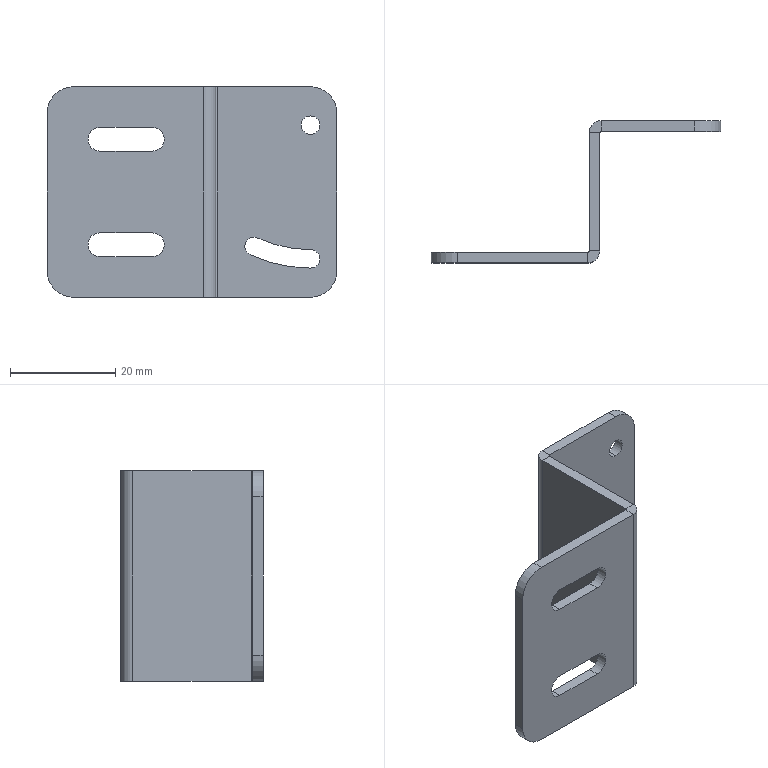Part | SolidWorks | features ICE 2, Fillet 1, FlatPattern 1, SMBaseFlange 1, SheetMetal 1 | 1 solid | 41 faces | box 55 x 27 x 40 mm | volume 5908 mm3 | plane 22 | cylinder 19 | commonest cylinder face diameters 3.5 x5 4.5 x4 10 x4 0.6 x2 4.6 x2 47.3 x1
STEP:
#1=CARTESIAN_POINT('',(20.,23.,30.95));
#2=VERTEX_POINT('',#1);
#3=CARTESIAN_POINT('',(20.,23.,34.45));
#4=VERTEX_POINT('',#3);
#5=CARTESIAN_POINT('',(20.,23.,32.7));
#6=DIRECTION('',(0.,1.,0.));
#7=DIRECTION('',(0.,0.,1.));
#8=AXIS2_PLACEMENT_3D('',#5,#6,#7);
#9=CIRCLE('',#8,1.75);
#10=EDGE_CURVE('',#2,#4,#9,.T.);
#11=ORIENTED_EDGE('',*,*,#10,.F.);
#12=CARTESIAN_POINT('',(20.,25.,30.95));
#13=VERTEX_POINT('',#12);
#14=CARTESIAN_POINT('',(20.,15.,30.95));
#15=DIRECTION('',(0.,1.,0.));
#16=VECTOR('',#15,1000.);
#17=LINE('',#14,#16);
#18=EDGE_CURVE('',#2,#13,#17,.T.);
#19=ORIENTED_EDGE('',*,*,#18,.T.);
#20=CARTESIAN_POINT('',(20.,25.,34.45));
#21=VERTEX_POINT('',#20);
#22=CARTESIAN_POINT('',(20.,25.,32.7));
#23=DIRECTION('',(0.,1.,0.));
#24=DIRECTION('',(0.,0.,1.));
#25=AXIS2_PLACEMENT_3D('',#22,#23,#24);
#26=CIRCLE('',#25,1.75);
#27=EDGE_CURVE('',#13,#21,#26,.T.);
#28=ORIENTED_EDGE('',*,*,#27,.T.);
#29=CARTESIAN_POINT('',(20.,15.,34.45));
#30=DIRECTION('',(0.,1.,0.));
#31=VECTOR('',#30,1000.);
#32=LINE('',#29,#31);
#33=EDGE_CURVE('',#4,#21,#32,.T.);
#34=ORIENTED_EDGE('',*,*,#33,.F.);
#35=EDGE_LOOP('',(#11,#19,#28,#34));
#36=FACE_OUTER_BOUND('',#35,.T.);
#37=CARTESIAN_POINT('',(20.,15.,32.7));
#38=DIRECTION('',(0.,1.,0.));
#39=DIRECTION('',(0.,0.,1.));
#40=AXIS2_PLACEMENT_3D('',#37,#38,#39);
#41=CYLINDRICAL_SURFACE('',#40,1.75);
#42=ADVANCED_FACE('',(#36),#41,.F.);
#43=CARTESIAN_POINT('',(9.265,23.,11.43));
#44=VERTEX_POINT('',#43);
#45=CARTESIAN_POINT('',(10.005,23.,11.266));
#46=VERTEX_POINT('',#45);
#47=CARTESIAN_POINT('',(9.265,23.,9.68));
#48=DIRECTION('',(0.,1.,0.));
#49=DIRECTION('',(0.,0.,1.));
#50=AXIS2_PLACEMENT_3D('',#47,#48,#49);
#51=CIRCLE('',#50,1.75);
#52=EDGE_CURVE('',#44,#46,#51,.T.);
#53=ORIENTED_EDGE('',*,*,#52,.F.);
#54=CARTESIAN_POINT('',(9.265,25.,11.43));
#55=VERTEX_POINT('',#54);
#56=CARTESIAN_POINT('',(9.265,15.,11.43));
#57=DIRECTION('',(0.,1.,0.));
#58=VECTOR('',#57,1000.);
#59=LINE('',#56,#58);
#60=EDGE_CURVE('',#44,#55,#59,.T.);
#61=ORIENTED_EDGE('',*,*,#60,.T.);
#62=CARTESIAN_POINT('',(10.005,25.,11.266));
#63=VERTEX_POINT('',#62);
#64=CARTESIAN_POINT('',(9.265,25.,9.68));
#65=DIRECTION('',(0.,1.,0.));
#66=DIRECTION('',(0.,0.,1.));
#67=AXIS2_PLACEMENT_3D('',#64,#65,#66);
#68=CIRCLE('',#67,1.75);
#69=EDGE_CURVE('',#55,#63,#68,.T.);
#70=ORIENTED_EDGE('',*,*,#69,.T.);
#71=CARTESIAN_POINT('',(10.005,15.,11.266));
#72=DIRECTION('',(0.,1.,0.));
#73=VECTOR('',#72,1000.);
#74=LINE('',#71,#73);
#75=EDGE_CURVE('',#46,#63,#74,.T.);
#76=ORIENTED_EDGE('',*,*,#75,.F.);
#77=EDGE_LOOP('',(#53,#61,#70,#76));
#78=FACE_OUTER_BOUND('',#77,.T.);
#79=CARTESIAN_POINT('',(9.265,15.,9.68));
#80=DIRECTION('',(0.,1.,0.));
#81=DIRECTION('',(0.,0.,1.));
#82=AXIS2_PLACEMENT_3D('',#79,#80,#81);
#83=CYLINDRICAL_SURFACE('',#82,1.75);
#84=ADVANCED_FACE('',(#78),#83,.F.);
#85=CARTESIAN_POINT('',(0.,0.3,40.));
#86=VERTEX_POINT('',#85);
#87=CARTESIAN_POINT('',(2.,0.3,40.));
#88=VERTEX_POINT('',#87);
#89=CARTESIAN_POINT('',(0.,0.3,40.));
#90=DIRECTION('',(1.,0.,0.));
#91=VECTOR('',#90,1000.);
#92=LINE('',#89,#91);
#93=EDGE_CURVE('',#86,#88,#92,.T.);
#94=ORIENTED_EDGE('',*,*,#93,.F.);
#95=CARTESIAN_POINT('',(-0.3,0.,40.));
#96=VERTEX_POINT('',#95);
#97=CARTESIAN_POINT('',(-0.3,0.3,40.));
#98=DIRECTION('',(0.,0.,1.));
#99=DIRECTION('',(-1.,0.,0.));
#100=AXIS2_PLACEMENT_3D('',#97,#98,#99);
#101=CIRCLE('',#100,0.3);
#102=EDGE_CURVE('',#96,#86,#101,.T.);
#103=ORIENTED_EDGE('',*,*,#102,.F.);
#104=CARTESIAN_POINT('',(-0.3,-2.,40.));
#105=VERTEX_POINT('',#104);
#106=CARTESIAN_POINT('',(-0.3,-2.,40.));
#107=DIRECTION('',(0.,1.,0.));
#108=VECTOR('',#107,1000.);
#109=LINE('',#106,#108);
#110=EDGE_CURVE('',#105,#96,#109,.T.);
#111=ORIENTED_EDGE('',*,*,#110,.F.);
#112=CARTESIAN_POINT('',(-0.3,0.3,40.));
#113=DIRECTION('',(0.,0.,1.));
#114=DIRECTION('',(1.,0.,0.));
#115=AXIS2_PLACEMENT_3D('',#112,#113,#114);
#116=CIRCLE('',#115,2.3);
#117=EDGE_CURVE('',#105,#88,#116,.T.);
#118=ORIENTED_EDGE('',*,*,#117,.T.);
#119=EDGE_LOOP('',(#94,#103,#111,#118));
#120=FACE_OUTER_BOUND('',#119,.T.);
#121=CARTESIAN_POINT('',(0.,0.3,40.));
#122=DIRECTION('',(0.,0.,1.));
#123=DIRECTION('',(1.,0.,0.));
#124=AXIS2_PLACEMENT_3D('',#121,#122,#123);
#125=PLANE('',#124);
#126=ADVANCED_FACE('',(#120),#125,.T.);
#127=CARTESIAN_POINT('',(0.,22.7,40.));
#128=VERTEX_POINT('',#127);
#129=CARTESIAN_POINT('',(0.,0.,40.));
#130=DIRECTION('',(0.,1.,0.));
#131=VECTOR('',#130,1000.);
#132=LINE('',#129,#131);
#133=EDGE_CURVE('',#86,#128,#132,.T.);
#134=ORIENTED_EDGE('',*,*,#133,.F.);
#135=ORIENTED_EDGE('',*,*,#93,.T.);
#136=CARTESIAN_POINT('',(2.,22.7,40.));
#137=VERTEX_POINT('',#136);
#138=CARTESIAN_POINT('',(2.,0.,40.));
#139=DIRECTION('',(0.,1.,0.));
#140=VECTOR('',#139,1000.);
#141=LINE('',#138,#140);
#142=EDGE_CURVE('',#88,#137,#141,.T.);
#143=ORIENTED_EDGE('',*,*,#142,.T.);
#144=CARTESIAN_POINT('',(2.,22.7,40.));
#145=DIRECTION('',(-1.,0.,0.));
#146=VECTOR('',#145,1000.);
#147=LINE('',#144,#146);
#148=EDGE_CURVE('',#137,#128,#147,.T.);
#149=ORIENTED_EDGE('',*,*,#148,.T.);
#150=EDGE_LOOP('',(#134,#135,#143,#149));
#151=FACE_OUTER_BOUND('',#150,.T.);
#152=CARTESIAN_POINT('',(-0.3,-2.,40.));
#153=DIRECTION('',(0.,0.,1.));
#154=DIRECTION('',(1.,0.,0.));
#155=AXIS2_PLACEMENT_3D('',#152,#153,#154);
#156=PLANE('',#155);
#157=ADVANCED_FACE('',(#151),#156,.T.);
#158=CARTESIAN_POINT('',(-0.3,0.,0.));
#159=VERTEX_POINT('',#158);
#160=CARTESIAN_POINT('',(-0.3,-2.,0.));
#161=VERTEX_POINT('',#160);
#162=CARTESIAN_POINT('',(-0.3,0.,0.));
#163=DIRECTION('',(0.,-1.,0.));
#164=VECTOR('',#163,1000.);
#165=LINE('',#162,#164);
#166=EDGE_CURVE('',#159,#161,#165,.T.);
#167=ORIENTED_EDGE('',*,*,#166,.F.);
#168=CARTESIAN_POINT('',(0.,0.3,0.));
#169=VERTEX_POINT('',#168);
#170=CARTESIAN_POINT('',(-0.3,0.3,0.));
#171=DIRECTION('',(0.,0.,1.));
#172=DIRECTION('',(-1.,0.,0.));
#173=AXIS2_PLACEMENT_3D('',#170,#171,#172);
#174=CIRCLE('',#173,0.3);
#175=EDGE_CURVE('',#159,#169,#174,.T.);
#176=ORIENTED_EDGE('',*,*,#175,.T.);
#177=CARTESIAN_POINT('',(2.,0.3,0.));
#178=VERTEX_POINT('',#177);
#179=CARTESIAN_POINT('',(2.,0.3,0.));
#180=DIRECTION('',(-1.,0.,0.));
#181=VECTOR('',#180,1000.);
#182=LINE('',#179,#181);
#183=EDGE_CURVE('',#178,#169,#182,.T.);
#184=ORIENTED_EDGE('',*,*,#183,.F.);
#185=CARTESIAN_POINT('',(-0.3,0.3,0.));
#186=DIRECTION('',(0.,0.,1.));
#187=DIRECTION('',(1.,0.,0.));
#188=AXIS2_PLACEMENT_3D('',#185,#186,#187);
#189=CIRCLE('',#188,2.3);
#190=EDGE_CURVE('',#161,#178,#189,.T.);
#191=ORIENTED_EDGE('',*,*,#190,.F.);
#192=EDGE_LOOP('',(#167,#176,#184,#191));
#193=FACE_OUTER_BOUND('',#192,.T.);
#194=CARTESIAN_POINT('',(-0.3,0.,0.));
#195=DIRECTION('',(0.,0.,-1.));
#196=DIRECTION('',(-1.,0.,0.));
#197=AXIS2_PLACEMENT_3D('',#194,#195,#196);
#198=PLANE('',#197);
#199=ADVANCED_FACE('',(#193),#198,.T.);
#200=CARTESIAN_POINT('',(-25.,-2.,0.));
#201=VERTEX_POINT('',#200);
#202=CARTESIAN_POINT('',(-30.,-2.,0.));
#203=DIRECTION('',(1.,0.,0.));
#204=VECTOR('',#203,1000.);
#205=LINE('',#202,#204);
#206=EDGE_CURVE('',#201,#161,#205,.T.);
#207=ORIENTED_EDGE('',*,*,#206,.F.);
#208=CARTESIAN_POINT('',(-25.,0.,0.));
#209=VERTEX_POINT('',#208);
#210=CARTESIAN_POINT('',(-25.,0.3,0.));
#211=DIRECTION('',(0.,1.,0.));
#212=VECTOR('',#211,1000.);
#213=LINE('',#210,#212);
#214=EDGE_CURVE('',#201,#209,#213,.T.);
#215=ORIENTED_EDGE('',*,*,#214,.T.);
#216=CARTESIAN_POINT('',(-30.,0.,0.));
#217=DIRECTION('',(1.,0.,0.));
#218=VECTOR('',#217,1000.);
#219=LINE('',#216,#218);
#220=EDGE_CURVE('',#209,#159,#219,.T.);
#221=ORIENTED_EDGE('',*,*,#220,.T.);
#222=ORIENTED_EDGE('',*,*,#166,.T.);
#223=EDGE_LOOP('',(#207,#215,#221,#222));
#224=FACE_OUTER_BOUND('',#223,.T.);
#225=CARTESIAN_POINT('',(2.,0.3,0.));
#226=DIRECTION('',(0.,0.,-1.));
#227=DIRECTION('',(-1.,0.,0.));
#228=AXIS2_PLACEMENT_3D('',#225,#226,#227);
#229=PLANE('',#228);
#230=ADVANCED_FACE('',(#224),#229,.T.);
#231=CARTESIAN_POINT('',(2.3,25.,40.));
#232=VERTEX_POINT('',#231);
#233=CARTESIAN_POINT('',(2.3,23.,40.));
#234=VERTEX_POINT('',#233);
#235=CARTESIAN_POINT('',(2.3,25.,40.));
#236=DIRECTION('',(0.,-1.,0.));
#237=VECTOR('',#236,1000.);
#238=LINE('',#235,#237);
#239=EDGE_CURVE('',#232,#234,#238,.T.);
#240=ORIENTED_EDGE('',*,*,#239,.F.);
#241=CARTESIAN_POINT('',(2.3,22.7,40.));
#242=DIRECTION('',(0.,0.,-1.));
#243=DIRECTION('',(1.,0.,0.));
#244=AXIS2_PLACEMENT_3D('',#241,#242,#243);
#245=CIRCLE('',#244,2.3);
#246=EDGE_CURVE('',#128,#232,#245,.T.);
#247=ORIENTED_EDGE('',*,*,#246,.F.);
#248=ORIENTED_EDGE('',*,*,#148,.F.);
#249=CARTESIAN_POINT('',(2.3,22.7,40.));
#250=DIRECTION('',(0.,0.,-1.));
#251=DIRECTION('',(1.,0.,0.));
#252=AXIS2_PLACEMENT_3D('',#249,#250,#251);
#253=CIRCLE('',#252,0.3);
#254=EDGE_CURVE('',#137,#234,#253,.T.);
#255=ORIENTED_EDGE('',*,*,#254,.T.);
#256=EDGE_LOOP('',(#240,#247,#248,#255));
#257=FACE_OUTER_BOUND('',#256,.T.);
#258=CARTESIAN_POINT('',(2.3,25.,40.));
#259=DIRECTION('',(0.,0.,1.));
#260=DIRECTION('',(1.,0.,0.));
#261=AXIS2_PLACEMENT_3D('',#258,#259,#260);
#262=PLANE('',#261);
#263=ADVANCED_FACE('',(#257),#262,.T.);
#264=CARTESIAN_POINT('',(20.,23.,40.));
#265=VERTEX_POINT('',#264);
#266=CARTESIAN_POINT('',(0.,23.,40.));
#267=DIRECTION('',(1.,0.,0.));
#268=VECTOR('',#267,1000.);
#269=LINE('',#266,#268);
#270=EDGE_CURVE('',#234,#265,#269,.T.);
#271=ORIENTED_EDGE('',*,*,#270,.T.);
#272=CARTESIAN_POINT('',(20.,25.,40.));
#273=VERTEX_POINT('',#272);
#274=CARTESIAN_POINT('',(20.,22.7,40.));
#275=DIRECTION('',(0.,1.,0.));
#276=VECTOR('',#275,1000.);
#277=LINE('',#274,#276);
#278=EDGE_CURVE('',#265,#273,#277,.T.);
#279=ORIENTED_EDGE('',*,*,#278,.T.);
#280=CARTESIAN_POINT('',(0.,25.,40.));
#281=DIRECTION('',(1.,0.,0.));
#282=VECTOR('',#281,1000.);
#283=LINE('',#280,#282);
#284=EDGE_CURVE('',#232,#273,#283,.T.);
#285=ORIENTED_EDGE('',*,*,#284,.F.);
#286=ORIENTED_EDGE('',*,*,#239,.T.);
#287=EDGE_LOOP('',(#271,#279,#285,#286));
#288=FACE_OUTER_BOUND('',#287,.T.);
#289=CARTESIAN_POINT('',(2.,22.7,40.));
#290=DIRECTION('',(0.,0.,1.));
#291=DIRECTION('',(1.,0.,0.));
#292=AXIS2_PLACEMENT_3D('',#289,#290,#291);
#293=PLANE('',#292);
#294=ADVANCED_FACE('',(#288),#293,.T.);
#295=CARTESIAN_POINT('',(0.,22.7,0.));
#296=VERTEX_POINT('',#295);
#297=CARTESIAN_POINT('',(2.,22.7,0.));
#298=VERTEX_POINT('',#297);
#299=CARTESIAN_POINT('',(0.,22.7,0.));
#300=DIRECTION('',(1.,0.,0.));
#301=VECTOR('',#300,1000.);
#302=LINE('',#299,#301);
#303=EDGE_CURVE('',#296,#298,#302,.T.);
#304=ORIENTED_EDGE('',*,*,#303,.F.);
#305=CARTESIAN_POINT('',(2.3,25.,0.));
#306=VERTEX_POINT('',#305);
#307=CARTESIAN_POINT('',(2.3,22.7,0.));
#308=DIRECTION('',(0.,0.,-1.));
#309=DIRECTION('',(1.,0.,0.));
#310=AXIS2_PLACEMENT_3D('',#307,#308,#309);
#311=CIRCLE('',#310,2.3);
#312=EDGE_CURVE('',#296,#306,#311,.T.);
#313=ORIENTED_EDGE('',*,*,#312,.T.);
#314=CARTESIAN_POINT('',(2.3,23.,0.));
#315=VERTEX_POINT('',#314);
#316=CARTESIAN_POINT('',(2.3,23.,0.));
#317=DIRECTION('',(0.,1.,0.));
#318=VECTOR('',#317,1000.);
#319=LINE('',#316,#318);
#320=EDGE_CURVE('',#315,#306,#319,.T.);
#321=ORIENTED_EDGE('',*,*,#320,.F.);
#322=CARTESIAN_POINT('',(2.3,22.7,0.));
#323=DIRECTION('',(0.,0.,-1.));
#324=DIRECTION('',(1.,0.,0.));
#325=AXIS2_PLACEMENT_3D('',#322,#323,#324);
#326=CIRCLE('',#325,0.3);
#327=EDGE_CURVE('',#298,#315,#326,.T.);
#328=ORIENTED_EDGE('',*,*,#327,.F.);
#329=EDGE_LOOP('',(#304,#313,#321,#328));
#330=FACE_OUTER_BOUND('',#329,.T.);
#331=CARTESIAN_POINT('',(0.,22.7,0.));
#332=DIRECTION('',(0.,0.,-1.));
#333=DIRECTION('',(-1.,0.,0.));
#334=AXIS2_PLACEMENT_3D('',#331,#332,#333);
#335=PLANE('',#334);
#336=ADVANCED_FACE('',(#330),#335,.T.);
#337=CARTESIAN_POINT('',(0.,0.,0.));
#338=DIRECTION('',(0.,1.,0.));
#339=VECTOR('',#338,1000.);
#340=LINE('',#337,#339);
#341=EDGE_CURVE('',#169,#296,#340,.T.);
#342=ORIENTED_EDGE('',*,*,#341,.T.);
#343=ORIENTED_EDGE('',*,*,#303,.T.);
#344=CARTESIAN_POINT('',(2.,0.,0.));
#345=DIRECTION('',(0.,1.,0.));
#346=VECTOR('',#345,1000.);
#347=LINE('',#344,#346);
#348=EDGE_CURVE('',#178,#298,#347,.T.);
#349=ORIENTED_EDGE('',*,*,#348,.F.);
#350=ORIENTED_EDGE('',*,*,#183,.T.);
#351=EDGE_LOOP('',(#342,#343,#349,#350));
#352=FACE_OUTER_BOUND('',#351,.T.);
#353=CARTESIAN_POINT('',(2.3,23.,0.));
#354=DIRECTION('',(0.,0.,-1.));
#355=DIRECTION('',(-1.,0.,0.));
#356=AXIS2_PLACEMENT_3D('',#353,#354,#355);
#357=PLANE('',#356);
#358=ADVANCED_FACE('',(#352),#357,.T.);
#359=CARTESIAN_POINT('',(20.,23.,32.7));
#360=DIRECTION('',(0.,1.,0.));
#361=DIRECTION('',(0.,0.,1.));
#362=AXIS2_PLACEMENT_3D('',#359,#360,#361);
#363=CIRCLE('',#362,1.75);
#364=EDGE_CURVE('',#4,#2,#363,.T.);
#365=ORIENTED_EDGE('',*,*,#364,.T.);
#366=ORIENTED_EDGE('',*,*,#10,.T.);
#367=EDGE_LOOP('',(#365,#366));
#368=FACE_BOUND('',#367,.T.);
#369=CARTESIAN_POINT('',(20.,23.,9.05));
#370=VERTEX_POINT('',#369);
#371=CARTESIAN_POINT('',(20.,23.,32.7));
#372=DIRECTION('',(0.,-1.,0.));
#373=DIRECTION('',(0.,0.,1.));
#374=AXIS2_PLACEMENT_3D('',#371,#372,#373);
#375=CIRCLE('',#374,23.65);
#376=EDGE_CURVE('',#46,#370,#375,.T.);
#377=ORIENTED_EDGE('',*,*,#376,.T.);
#378=CARTESIAN_POINT('',(20.,23.,5.55));
#379=VERTEX_POINT('',#378);
#380=CARTESIAN_POINT('',(20.,23.,7.3));
#381=DIRECTION('',(0.,1.,0.));
#382=DIRECTION('',(0.,0.,1.));
#383=AXIS2_PLACEMENT_3D('',#380,#381,#382);
#384=CIRCLE('',#383,1.75);
#385=EDGE_CURVE('',#370,#379,#384,.T.);
#386=ORIENTED_EDGE('',*,*,#385,.T.);
#387=CARTESIAN_POINT('',(8.526,23.,8.094));
#388=VERTEX_POINT('',#387);
#389=CARTESIAN_POINT('',(20.,23.,32.7));
#390=DIRECTION('',(0.,1.,0.));
#391=DIRECTION('',(0.,0.,1.));
#392=AXIS2_PLACEMENT_3D('',#389,#390,#391);
#393=CIRCLE('',#392,27.15);
#394=EDGE_CURVE('',#379,#388,#393,.T.);
#395=ORIENTED_EDGE('',*,*,#394,.T.);
#396=CARTESIAN_POINT('',(9.265,23.,9.68));
#397=DIRECTION('',(0.,1.,0.));
#398=DIRECTION('',(0.,0.,1.));
#399=AXIS2_PLACEMENT_3D('',#396,#397,#398);
#400=CIRCLE('',#399,1.75);
#401=EDGE_CURVE('',#388,#44,#400,.T.);
#402=ORIENTED_EDGE('',*,*,#401,.T.);
#403=ORIENTED_EDGE('',*,*,#52,.T.);
#404=EDGE_LOOP('',(#377,#386,#395,#402,#403));
#405=FACE_BOUND('',#404,.T.);
#406=CARTESIAN_POINT('',(25.,23.,35.));
#407=VERTEX_POINT('',#406);
#408=CARTESIAN_POINT('',(25.,23.,5.));
#409=VERTEX_POINT('',#408);
#410=CARTESIAN_POINT('',(25.,23.,40.));
#411=DIRECTION('',(0.,0.,-1.));
#412=VECTOR('',#411,1000.);
#413=LINE('',#410,#412);
#414=EDGE_CURVE('',#407,#409,#413,.T.);
#415=ORIENTED_EDGE('',*,*,#414,.F.);
#416=CARTESIAN_POINT('',(20.,23.,35.));
#417=DIRECTION('',(0.,-1.,0.));
#418=DIRECTION('',(0.,0.,1.));
#419=AXIS2_PLACEMENT_3D('',#416,#417,#418);
#420=CIRCLE('',#419,5.);
#421=EDGE_CURVE('',#407,#265,#420,.T.);
#422=ORIENTED_EDGE('',*,*,#421,.T.);
#423=ORIENTED_EDGE('',*,*,#270,.F.);
#424=CARTESIAN_POINT('',(2.3,23.,40.));
#425=DIRECTION('',(0.,0.,-1.));
#426=VECTOR('',#425,1000.);
#427=LINE('',#424,#426);
#428=EDGE_CURVE('',#234,#315,#427,.T.);
#429=ORIENTED_EDGE('',*,*,#428,.T.);
#430=CARTESIAN_POINT('',(20.,23.,0.));
#431=VERTEX_POINT('',#430);
#432=CARTESIAN_POINT('',(0.,23.,0.));
#433=DIRECTION('',(1.,0.,0.));
#434=VECTOR('',#433,1000.);
#435=LINE('',#432,#434);
#436=EDGE_CURVE('',#315,#431,#435,.T.);
#437=ORIENTED_EDGE('',*,*,#436,.T.);
#438=CARTESIAN_POINT('',(20.,23.,5.));
#439=DIRECTION('',(0.,-1.,0.));
#440=DIRECTION('',(0.,0.,1.));
#441=AXIS2_PLACEMENT_3D('',#438,#439,#440);
#442=CIRCLE('',#441,5.);
#443=EDGE_CURVE('',#431,#409,#442,.T.);
#444=ORIENTED_EDGE('',*,*,#443,.T.);
#445=EDGE_LOOP('',(#415,#422,#423,#429,#437,#444));
#446=FACE_OUTER_BOUND('',#445,.T.);
#447=CARTESIAN_POINT('',(0.,23.,40.));
#448=DIRECTION('',(0.,1.,0.));
#449=DIRECTION('',(0.,0.,1.));
#450=AXIS2_PLACEMENT_3D('',#447,#448,#449);
#451=PLANE('',#450);
#452=ADVANCED_FACE('',(#368,#405,#446),#451,.F.);
#453=CARTESIAN_POINT('',(25.,25.,35.));
#454=VERTEX_POINT('',#453);
#455=CARTESIAN_POINT('',(25.,25.,5.));
#456=VERTEX_POINT('',#455);
#457=CARTESIAN_POINT('',(25.,25.,40.));
#458=DIRECTION('',(0.,0.,-1.));
#459=VECTOR('',#458,1000.);
#460=LINE('',#457,#459);
#461=EDGE_CURVE('',#454,#456,#460,.T.);
#462=ORIENTED_EDGE('',*,*,#461,.F.);
#463=CARTESIAN_POINT('',(25.,25.,35.));
#464=DIRECTION('',(0.,-1.,0.));
#465=VECTOR('',#464,1000.);
#466=LINE('',#463,#465);
#467=EDGE_CURVE('',#454,#407,#466,.T.);
#468=ORIENTED_EDGE('',*,*,#467,.T.);
#469=ORIENTED_EDGE('',*,*,#414,.T.);
#470=CARTESIAN_POINT('',(25.,25.,5.));
#471=DIRECTION('',(0.,1.,0.));
#472=VECTOR('',#471,1000.);
#473=LINE('',#470,#472);
#474=EDGE_CURVE('',#409,#456,#473,.T.);
#475=ORIENTED_EDGE('',*,*,#474,.T.);
#476=EDGE_LOOP('',(#462,#468,#469,#475));
#477=FACE_OUTER_BOUND('',#476,.T.);
#478=CARTESIAN_POINT('',(25.,25.,40.));
#479=DIRECTION('',(1.,0.,0.));
#480=DIRECTION('',(0.,0.,-1.));
#481=AXIS2_PLACEMENT_3D('',#478,#479,#480);
#482=PLANE('',#481);
#483=ADVANCED_FACE('',(#477),#482,.T.);
#484=CARTESIAN_POINT('',(20.,25.,32.7));
#485=DIRECTION('',(0.,1.,0.));
#486=DIRECTION('',(0.,0.,1.));
#487=AXIS2_PLACEMENT_3D('',#484,#485,#486);
#488=CIRCLE('',#487,1.75);
#489=EDGE_CURVE('',#21,#13,#488,.T.);
#490=ORIENTED_EDGE('',*,*,#489,.F.);
#491=ORIENTED_EDGE('',*,*,#27,.F.);
#492=EDGE_LOOP('',(#490,#491));
#493=FACE_BOUND('',#492,.T.);
#494=CARTESIAN_POINT('',(20.,25.,9.05));
#495=VERTEX_POINT('',#494);
#496=CARTESIAN_POINT('',(20.,25.,5.55));
#497=VERTEX_POINT('',#496);
#498=CARTESIAN_POINT('',(20.,25.,7.3));
#499=DIRECTION('',(0.,1.,0.));
#500=DIRECTION('',(0.,0.,1.));
#501=AXIS2_PLACEMENT_3D('',#498,#499,#500);
#502=CIRCLE('',#501,1.75);
#503=EDGE_CURVE('',#495,#497,#502,.T.);
#504=ORIENTED_EDGE('',*,*,#503,.F.);
#505=CARTESIAN_POINT('',(20.,25.,32.7));
#506=DIRECTION('',(0.,-1.,0.));
#507=DIRECTION('',(0.,0.,1.));
#508=AXIS2_PLACEMENT_3D('',#505,#506,#507);
#509=CIRCLE('',#508,23.65);
#510=EDGE_CURVE('',#63,#495,#509,.T.);
#511=ORIENTED_EDGE('',*,*,#510,.F.);
#512=ORIENTED_EDGE('',*,*,#69,.F.);
#513=CARTESIAN_POINT('',(8.526,25.,8.094));
#514=VERTEX_POINT('',#513);
#515=CARTESIAN_POINT('',(9.265,25.,9.68));
#516=DIRECTION('',(0.,1.,0.));
#517=DIRECTION('',(0.,0.,1.));
#518=AXIS2_PLACEMENT_3D('',#515,#516,#517);
#519=CIRCLE('',#518,1.75);
#520=EDGE_CURVE('',#514,#55,#519,.T.);
#521=ORIENTED_EDGE('',*,*,#520,.F.);
#522=CARTESIAN_POINT('',(20.,25.,32.7));
#523=DIRECTION('',(0.,1.,0.));
#524=DIRECTION('',(0.,0.,1.));
#525=AXIS2_PLACEMENT_3D('',#522,#523,#524);
#526=CIRCLE('',#525,27.15);
#527=EDGE_CURVE('',#497,#514,#526,.T.);
#528=ORIENTED_EDGE('',*,*,#527,.F.);
#529=EDGE_LOOP('',(#504,#511,#512,#521,#528));
#530=FACE_BOUND('',#529,.T.);
#531=ORIENTED_EDGE('',*,*,#284,.T.);
#532=CARTESIAN_POINT('',(20.,25.,35.));
#533=DIRECTION('',(0.,1.,0.));
#534=DIRECTION('',(0.,0.,1.));
#535=AXIS2_PLACEMENT_3D('',#532,#533,#534);
#536=CIRCLE('',#535,5.);
#537=EDGE_CURVE('',#273,#454,#536,.T.);
#538=ORIENTED_EDGE('',*,*,#537,.T.);
#539=ORIENTED_EDGE('',*,*,#461,.T.);
#540=CARTESIAN_POINT('',(20.,25.,0.));
#541=VERTEX_POINT('',#540);
#542=CARTESIAN_POINT('',(20.,25.,5.));
#543=DIRECTION('',(0.,1.,0.));
#544=DIRECTION('',(0.,0.,1.));
#545=AXIS2_PLACEMENT_3D('',#542,#543,#544);
#546=CIRCLE('',#545,5.);
#547=EDGE_CURVE('',#456,#541,#546,.T.);
#548=ORIENTED_EDGE('',*,*,#547,.T.);
#549=CARTESIAN_POINT('',(0.,25.,0.));
#550=DIRECTION('',(1.,0.,0.));
#551=VECTOR('',#550,1000.);
#552=LINE('',#549,#551);
#553=EDGE_CURVE('',#306,#541,#552,.T.);
#554=ORIENTED_EDGE('',*,*,#553,.F.);
#555=CARTESIAN_POINT('',(2.3,25.,40.));
#556=DIRECTION('',(0.,0.,-1.));
#557=VECTOR('',#556,1000.);
#558=LINE('',#555,#557);
#559=EDGE_CURVE('',#232,#306,#558,.T.);
#560=ORIENTED_EDGE('',*,*,#559,.F.);
#561=EDGE_LOOP('',(#531,#538,#539,#548,#554,#560));
#562=FACE_OUTER_BOUND('',#561,.T.);
#563=CARTESIAN_POINT('',(0.,25.,40.));
#564=DIRECTION('',(0.,1.,0.));
#565=DIRECTION('',(0.,0.,1.));
#566=AXIS2_PLACEMENT_3D('',#563,#564,#565);
#567=PLANE('',#566);
#568=ADVANCED_FACE('',(#493,#530,#562),#567,.T.);
#569=ORIENTED_EDGE('',*,*,#312,.F.);
#570=CARTESIAN_POINT('',(0.,22.7,40.));
#571=DIRECTION('',(0.,0.,-1.));
#572=VECTOR('',#571,1000.);
#573=LINE('',#570,#572);
#574=EDGE_CURVE('',#128,#296,#573,.T.);
#575=ORIENTED_EDGE('',*,*,#574,.F.);
#576=ORIENTED_EDGE('',*,*,#246,.T.);
#577=ORIENTED_EDGE('',*,*,#559,.T.);
#578=EDGE_LOOP('',(#569,#575,#576,#577));
#579=FACE_OUTER_BOUND('',#578,.T.);
#580=CARTESIAN_POINT('',(2.3,22.7,40.));
#581=DIRECTION('',(0.,0.,-1.));
#582=DIRECTION('',(-1.,0.,0.));
#583=AXIS2_PLACEMENT_3D('',#580,#581,#582);
#584=CYLINDRICAL_SURFACE('',#583,2.3);
#585=ADVANCED_FACE('',(#579),#584,.T.);
#586=ORIENTED_EDGE('',*,*,#341,.F.);
#587=CARTESIAN_POINT('',(0.,0.3,40.));
#588=DIRECTION('',(0.,0.,-1.));
#589=VECTOR('',#588,1000.);
#590=LINE('',#587,#589);
#591=EDGE_CURVE('',#86,#169,#590,.T.);
#592=ORIENTED_EDGE('',*,*,#591,.F.);
#593=ORIENTED_EDGE('',*,*,#133,.T.);
#594=ORIENTED_EDGE('',*,*,#574,.T.);
#595=EDGE_LOOP('',(#586,#592,#593,#594));
#596=FACE_OUTER_BOUND('',#595,.T.);
#597=CARTESIAN_POINT('',(0.,0.,40.));
#598=DIRECTION('',(-1.,0.,0.));
#599=DIRECTION('',(0.,0.,1.));
#600=AXIS2_PLACEMENT_3D('',#597,#598,#599);
#601=PLANE('',#600);
#602=ADVANCED_FACE('',(#596),#601,.T.);
#603=ORIENTED_EDGE('',*,*,#175,.F.);
#604=CARTESIAN_POINT('',(-0.3,0.,40.));
#605=DIRECTION('',(0.,0.,-1.));
#606=VECTOR('',#605,1000.);
#607=LINE('',#604,#606);
#608=EDGE_CURVE('',#96,#159,#607,.T.);
#609=ORIENTED_EDGE('',*,*,#608,.F.);
#610=ORIENTED_EDGE('',*,*,#102,.T.);
#611=ORIENTED_EDGE('',*,*,#591,.T.);
#612=EDGE_LOOP('',(#603,#609,#610,#611));
#613=FACE_OUTER_BOUND('',#612,.T.);
#614=CARTESIAN_POINT('',(-0.3,0.3,40.));
#615=DIRECTION('',(0.,0.,-1.));
#616=DIRECTION('',(-1.,0.,0.));
#617=AXIS2_PLACEMENT_3D('',#614,#615,#616);
#618=CYLINDRICAL_SURFACE('',#617,0.3);
#619=ADVANCED_FACE('',(#613),#618,.F.);
#620=CARTESIAN_POINT('',(-20.,0.,7.75));
#621=VERTEX_POINT('',#620);
#622=CARTESIAN_POINT('',(-20.,0.,12.25));
#623=VERTEX_POINT('',#622);
#624=CARTESIAN_POINT('',(-20.,0.,10.));
#625=DIRECTION('',(0.,1.,0.));
#626=DIRECTION('',(0.,0.,1.));
#627=AXIS2_PLACEMENT_3D('',#624,#625,#626);
#628=CIRCLE('',#627,2.25);
#629=EDGE_CURVE('',#621,#623,#628,.T.);
#630=ORIENTED_EDGE('',*,*,#629,.F.);
#631=CARTESIAN_POINT('',(-10.,0.,7.75));
#632=VERTEX_POINT('',#631);
#633=CARTESIAN_POINT('',(-20.,0.,7.75));
#634=DIRECTION('',(-1.,0.,0.));
#635=VECTOR('',#634,1000.);
#636=LINE('',#633,#635);
#637=EDGE_CURVE('',#632,#621,#636,.T.);
#638=ORIENTED_EDGE('',*,*,#637,.F.);
#639=CARTESIAN_POINT('',(-10.,0.,12.25));
#640=VERTEX_POINT('',#639);
#641=CARTESIAN_POINT('',(-10.,0.,10.));
#642=DIRECTION('',(0.,1.,0.));
#643=DIRECTION('',(0.,0.,1.));
#644=AXIS2_PLACEMENT_3D('',#641,#642,#643);
#645=CIRCLE('',#644,2.25);
#646=EDGE_CURVE('',#640,#632,#645,.T.);
#647=ORIENTED_EDGE('',*,*,#646,.F.);
#648=CARTESIAN_POINT('',(-20.,0.,12.25));
#649=DIRECTION('',(1.,0.,0.));
#650=VECTOR('',#649,1000.);
#651=LINE('',#648,#650);
#652=EDGE_CURVE('',#623,#640,#651,.T.);
#653=ORIENTED_EDGE('',*,*,#652,.F.);
#654=EDGE_LOOP('',(#630,#638,#647,#653));
#655=FACE_BOUND('',#654,.T.);
#656=CARTESIAN_POINT('',(-20.,0.,27.75));
#657=VERTEX_POINT('',#656);
#658=CARTESIAN_POINT('',(-20.,0.,32.25));
#659=VERTEX_POINT('',#658);
#660=CARTESIAN_POINT('',(-20.,0.,30.));
#661=DIRECTION('',(0.,1.,0.));
#662=DIRECTION('',(0.,0.,1.));
#663=AXIS2_PLACEMENT_3D('',#660,#661,#662);
#664=CIRCLE('',#663,2.25);
#665=EDGE_CURVE('',#657,#659,#664,.T.);
#666=ORIENTED_EDGE('',*,*,#665,.F.);
#667=CARTESIAN_POINT('',(-10.,0.,27.75));
#668=VERTEX_POINT('',#667);
#669=CARTESIAN_POINT('',(-20.,0.,27.75));
#670=DIRECTION('',(-1.,0.,0.));
#671=VECTOR('',#670,1000.);
#672=LINE('',#669,#671);
#673=EDGE_CURVE('',#668,#657,#672,.T.);
#674=ORIENTED_EDGE('',*,*,#673,.F.);
#675=CARTESIAN_POINT('',(-10.,0.,32.25));
#676=VERTEX_POINT('',#675);
#677=CARTESIAN_POINT('',(-10.,0.,30.));
#678=DIRECTION('',(0.,1.,0.));
#679=DIRECTION('',(0.,0.,1.));
#680=AXIS2_PLACEMENT_3D('',#677,#678,#679);
#681=CIRCLE('',#680,2.25);
#682=EDGE_CURVE('',#676,#668,#681,.T.);
#683=ORIENTED_EDGE('',*,*,#682,.F.);
#684=CARTESIAN_POINT('',(-20.,0.,32.25));
#685=DIRECTION('',(1.,0.,0.));
#686=VECTOR('',#685,1000.);
#687=LINE('',#684,#686);
#688=EDGE_CURVE('',#659,#676,#687,.T.);
#689=ORIENTED_EDGE('',*,*,#688,.F.);
#690=EDGE_LOOP('',(#666,#674,#683,#689));
#691=FACE_BOUND('',#690,.T.);
#692=CARTESIAN_POINT('',(-30.,0.,35.));
#693=VERTEX_POINT('',#692);
#694=CARTESIAN_POINT('',(-30.,0.,5.));
#695=VERTEX_POINT('',#694);
#696=CARTESIAN_POINT('',(-30.,0.,40.));
#697=DIRECTION('',(0.,0.,-1.));
#698=VECTOR('',#697,1000.);
#699=LINE('',#696,#698);
#700=EDGE_CURVE('',#693,#695,#699,.T.);
#701=ORIENTED_EDGE('',*,*,#700,.F.);
#702=CARTESIAN_POINT('',(-25.,0.,40.));
#703=VERTEX_POINT('',#702);
#704=CARTESIAN_POINT('',(-25.,0.,35.));
#705=DIRECTION('',(0.,1.,0.));
#706=DIRECTION('',(0.,0.,1.));
#707=AXIS2_PLACEMENT_3D('',#704,#705,#706);
#708=CIRCLE('',#707,5.);
#709=EDGE_CURVE('',#693,#703,#708,.T.);
#710=ORIENTED_EDGE('',*,*,#709,.T.);
#711=CARTESIAN_POINT('',(-30.,0.,40.));
#712=DIRECTION('',(1.,0.,0.));
#713=VECTOR('',#712,1000.);
#714=LINE('',#711,#713);
#715=EDGE_CURVE('',#703,#96,#714,.T.);
#716=ORIENTED_EDGE('',*,*,#715,.T.);
#717=ORIENTED_EDGE('',*,*,#608,.T.);
#718=ORIENTED_EDGE('',*,*,#220,.F.);
#719=CARTESIAN_POINT('',(-25.,0.,5.));
#720=DIRECTION('',(0.,1.,0.));
#721=DIRECTION('',(0.,0.,1.));
#722=AXIS2_PLACEMENT_3D('',#719,#720,#721);
#723=CIRCLE('',#722,5.);
#724=EDGE_CURVE('',#209,#695,#723,.T.);
#725=ORIENTED_EDGE('',*,*,#724,.T.);
#726=EDGE_LOOP('',(#701,#710,#716,#717,#718,#725));
#727=FACE_OUTER_BOUND('',#726,.T.);
#728=CARTESIAN_POINT('',(-30.,0.,40.));
#729=DIRECTION('',(0.,1.,0.));
#730=DIRECTION('',(0.,0.,1.));
#731=AXIS2_PLACEMENT_3D('',#728,#729,#730);
#732=PLANE('',#731);
#733=ADVANCED_FACE('',(#655,#691,#727),#732,.T.);
#734=CARTESIAN_POINT('',(-30.,-2.,35.));
#735=VERTEX_POINT('',#734);
#736=CARTESIAN_POINT('',(-30.,-2.,5.));
#737=VERTEX_POINT('',#736);
#738=CARTESIAN_POINT('',(-30.,-2.,40.));
#739=DIRECTION('',(0.,0.,-1.));
#740=VECTOR('',#739,1000.);
#741=LINE('',#738,#740);
#742=EDGE_CURVE('',#735,#737,#741,.T.);
#743=ORIENTED_EDGE('',*,*,#742,.F.);
#744=CARTESIAN_POINT('',(-30.,-2.,35.));
#745=DIRECTION('',(0.,1.,0.));
#746=VECTOR('',#745,1000.);
#747=LINE('',#744,#746);
#748=EDGE_CURVE('',#735,#693,#747,.T.);
#749=ORIENTED_EDGE('',*,*,#748,.T.);
#750=ORIENTED_EDGE('',*,*,#700,.T.);
#751=CARTESIAN_POINT('',(-30.,-2.,5.));
#752=DIRECTION('',(0.,-1.,0.));
#753=VECTOR('',#752,1000.);
#754=LINE('',#751,#753);
#755=EDGE_CURVE('',#695,#737,#754,.T.);
#756=ORIENTED_EDGE('',*,*,#755,.T.);
#757=EDGE_LOOP('',(#743,#749,#750,#756));
#758=FACE_OUTER_BOUND('',#757,.T.);
#759=CARTESIAN_POINT('',(-30.,-2.,40.));
#760=DIRECTION('',(-1.,0.,0.));
#761=DIRECTION('',(0.,0.,1.));
#762=AXIS2_PLACEMENT_3D('',#759,#760,#761);
#763=PLANE('',#762);
#764=ADVANCED_FACE('',(#758),#763,.T.);
#765=CARTESIAN_POINT('',(-10.,-2.,7.75));
#766=VERTEX_POINT('',#765);
#767=CARTESIAN_POINT('',(-20.,-2.,7.75));
#768=VERTEX_POINT('',#767);
#769=CARTESIAN_POINT('',(-30.,-2.,7.75));
#770=DIRECTION('',(-1.,0.,0.));
#771=VECTOR('',#770,1000.);
#772=LINE('',#769,#771);
#773=EDGE_CURVE('',#766,#768,#772,.T.);
#774=ORIENTED_EDGE('',*,*,#773,.T.);
#775=CARTESIAN_POINT('',(-20.,-2.,12.25));
#776=VERTEX_POINT('',#775);
#777=CARTESIAN_POINT('',(-20.,-2.,10.));
#778=DIRECTION('',(0.,1.,0.));
#779=DIRECTION('',(0.,0.,1.));
#780=AXIS2_PLACEMENT_3D('',#777,#778,#779);
#781=CIRCLE('',#780,2.25);
#782=EDGE_CURVE('',#768,#776,#781,.T.);
#783=ORIENTED_EDGE('',*,*,#782,.T.);
#784=CARTESIAN_POINT('',(-10.,-2.,12.25));
#785=VERTEX_POINT('',#784);
#786=CARTESIAN_POINT('',(-30.,-2.,12.25));
#787=DIRECTION('',(1.,0.,0.));
#788=VECTOR('',#787,1000.);
#789=LINE('',#786,#788);
#790=EDGE_CURVE('',#776,#785,#789,.T.);
#791=ORIENTED_EDGE('',*,*,#790,.T.);
#792=CARTESIAN_POINT('',(-10.,-2.,10.));
#793=DIRECTION('',(0.,1.,0.));
#794=DIRECTION('',(0.,0.,1.));
#795=AXIS2_PLACEMENT_3D('',#792,#793,#794);
#796=CIRCLE('',#795,2.25);
#797=EDGE_CURVE('',#785,#766,#796,.T.);
#798=ORIENTED_EDGE('',*,*,#797,.T.);
#799=EDGE_LOOP('',(#774,#783,#791,#798));
#800=FACE_BOUND('',#799,.T.);
#801=CARTESIAN_POINT('',(-10.,-2.,27.75));
#802=VERTEX_POINT('',#801);
#803=CARTESIAN_POINT('',(-20.,-2.,27.75));
#804=VERTEX_POINT('',#803);
#805=CARTESIAN_POINT('',(-30.,-2.,27.75));
#806=DIRECTION('',(-1.,0.,0.));
#807=VECTOR('',#806,1000.);
#808=LINE('',#805,#807);
#809=EDGE_CURVE('',#802,#804,#808,.T.);
#810=ORIENTED_EDGE('',*,*,#809,.T.);
#811=CARTESIAN_POINT('',(-20.,-2.,32.25));
#812=VERTEX_POINT('',#811);
#813=CARTESIAN_POINT('',(-20.,-2.,30.));
#814=DIRECTION('',(0.,1.,0.));
#815=DIRECTION('',(0.,0.,1.));
#816=AXIS2_PLACEMENT_3D('',#813,#814,#815);
#817=CIRCLE('',#816,2.25);
#818=EDGE_CURVE('',#804,#812,#817,.T.);
#819=ORIENTED_EDGE('',*,*,#818,.T.);
#820=CARTESIAN_POINT('',(-10.,-2.,32.25));
#821=VERTEX_POINT('',#820);
#822=CARTESIAN_POINT('',(-30.,-2.,32.25));
#823=DIRECTION('',(1.,0.,0.));
#824=VECTOR('',#823,1000.);
#825=LINE('',#822,#824);
#826=EDGE_CURVE('',#812,#821,#825,.T.);
#827=ORIENTED_EDGE('',*,*,#826,.T.);
#828=CARTESIAN_POINT('',(-10.,-2.,30.));
#829=DIRECTION('',(0.,1.,0.));
#830=DIRECTION('',(0.,0.,1.));
#831=AXIS2_PLACEMENT_3D('',#828,#829,#830);
#832=CIRCLE('',#831,2.25);
#833=EDGE_CURVE('',#821,#802,#832,.T.);
#834=ORIENTED_EDGE('',*,*,#833,.T.);
#835=EDGE_LOOP('',(#810,#819,#827,#834));
#836=FACE_BOUND('',#835,.T.);
#837=CARTESIAN_POINT('',(-25.,-2.,40.));
#838=VERTEX_POINT('',#837);
#839=CARTESIAN_POINT('',(-30.,-2.,40.));
#840=DIRECTION('',(1.,0.,0.));
#841=VECTOR('',#840,1000.);
#842=LINE('',#839,#841);
#843=EDGE_CURVE('',#838,#105,#842,.T.);
#844=ORIENTED_EDGE('',*,*,#843,.F.);
#845=CARTESIAN_POINT('',(-25.,-2.,35.));
#846=DIRECTION('',(0.,-1.,0.));
#847=DIRECTION('',(0.,0.,1.));
#848=AXIS2_PLACEMENT_3D('',#845,#846,#847);
#849=CIRCLE('',#848,5.);
#850=EDGE_CURVE('',#838,#735,#849,.T.);
#851=ORIENTED_EDGE('',*,*,#850,.T.);
#852=ORIENTED_EDGE('',*,*,#742,.T.);
#853=CARTESIAN_POINT('',(-25.,-2.,5.));
#854=DIRECTION('',(0.,-1.,0.));
#855=DIRECTION('',(0.,0.,1.));
#856=AXIS2_PLACEMENT_3D('',#853,#854,#855);
#857=CIRCLE('',#856,5.);
#858=EDGE_CURVE('',#737,#201,#857,.T.);
#859=ORIENTED_EDGE('',*,*,#858,.T.);
#860=ORIENTED_EDGE('',*,*,#206,.T.);
#861=CARTESIAN_POINT('',(-0.3,-2.,40.));
#862=DIRECTION('',(0.,0.,-1.));
#863=VECTOR('',#862,1000.);
#864=LINE('',#861,#863);
#865=EDGE_CURVE('',#105,#161,#864,.T.);
#866=ORIENTED_EDGE('',*,*,#865,.F.);
#867=EDGE_LOOP('',(#844,#851,#852,#859,#860,#866));
#868=FACE_OUTER_BOUND('',#867,.T.);
#869=CARTESIAN_POINT('',(-30.,-2.,40.));
#870=DIRECTION('',(0.,1.,0.));
#871=DIRECTION('',(0.,0.,1.));
#872=AXIS2_PLACEMENT_3D('',#869,#870,#871);
#873=PLANE('',#872);
#874=ADVANCED_FACE('',(#800,#836,#868),#873,.F.);
#875=ORIENTED_EDGE('',*,*,#190,.T.);
#876=CARTESIAN_POINT('',(2.,0.3,40.));
#877=DIRECTION('',(0.,0.,-1.));
#878=VECTOR('',#877,1000.);
#879=LINE('',#876,#878);
#880=EDGE_CURVE('',#88,#178,#879,.T.);
#881=ORIENTED_EDGE('',*,*,#880,.F.);
#882=ORIENTED_EDGE('',*,*,#117,.F.);
#883=ORIENTED_EDGE('',*,*,#865,.T.);
#884=EDGE_LOOP('',(#875,#881,#882,#883));
#885=FACE_OUTER_BOUND('',#884,.T.);
#886=CARTESIAN_POINT('',(-0.3,0.3,40.));
#887=DIRECTION('',(0.,0.,-1.));
#888=DIRECTION('',(-1.,0.,0.));
#889=AXIS2_PLACEMENT_3D('',#886,#887,#888);
#890=CYLINDRICAL_SURFACE('',#889,2.3);
#891=ADVANCED_FACE('',(#885),#890,.T.);
#892=ORIENTED_EDGE('',*,*,#348,.T.);
#893=CARTESIAN_POINT('',(2.,22.7,40.));
#894=DIRECTION('',(0.,0.,-1.));
#895=VECTOR('',#894,1000.);
#896=LINE('',#893,#895);
#897=EDGE_CURVE('',#137,#298,#896,.T.);
#898=ORIENTED_EDGE('',*,*,#897,.F.);
#899=ORIENTED_EDGE('',*,*,#142,.F.);
#900=ORIENTED_EDGE('',*,*,#880,.T.);
#901=EDGE_LOOP('',(#892,#898,#899,#900));
#902=FACE_OUTER_BOUND('',#901,.T.);
#903=CARTESIAN_POINT('',(2.,0.,40.));
#904=DIRECTION('',(-1.,0.,0.));
#905=DIRECTION('',(0.,0.,1.));
#906=AXIS2_PLACEMENT_3D('',#903,#904,#905);
#907=PLANE('',#906);
#908=ADVANCED_FACE('',(#902),#907,.F.);
#909=ORIENTED_EDGE('',*,*,#327,.T.);
#910=ORIENTED_EDGE('',*,*,#428,.F.);
#911=ORIENTED_EDGE('',*,*,#254,.F.);
#912=ORIENTED_EDGE('',*,*,#897,.T.);
#913=EDGE_LOOP('',(#909,#910,#911,#912));
#914=FACE_OUTER_BOUND('',#913,.T.);
#915=CARTESIAN_POINT('',(2.3,22.7,40.));
#916=DIRECTION('',(0.,0.,-1.));
#917=DIRECTION('',(-1.,0.,0.));
#918=AXIS2_PLACEMENT_3D('',#915,#916,#917);
#919=CYLINDRICAL_SURFACE('',#918,0.3);
#920=ADVANCED_FACE('',(#914),#919,.F.);
#921=ORIENTED_EDGE('',*,*,#715,.F.);
#922=CARTESIAN_POINT('',(-25.,22.7,40.));
#923=DIRECTION('',(0.,-1.,0.));
#924=VECTOR('',#923,1000.);
#925=LINE('',#922,#924);
#926=EDGE_CURVE('',#703,#838,#925,.T.);
#927=ORIENTED_EDGE('',*,*,#926,.T.);
#928=ORIENTED_EDGE('',*,*,#843,.T.);
#929=ORIENTED_EDGE('',*,*,#110,.T.);
#930=EDGE_LOOP('',(#921,#927,#928,#929));
#931=FACE_OUTER_BOUND('',#930,.T.);
#932=CARTESIAN_POINT('',(2.3,22.7,40.));
#933=DIRECTION('',(0.,0.,1.));
#934=DIRECTION('',(1.,0.,0.));
#935=AXIS2_PLACEMENT_3D('',#932,#933,#934);
#936=PLANE('',#935);
#937=ADVANCED_FACE('',(#931),#936,.T.);
#938=ORIENTED_EDGE('',*,*,#553,.T.);
#939=CARTESIAN_POINT('',(20.,23.,0.));
#940=DIRECTION('',(0.,-1.,0.));
#941=VECTOR('',#940,1000.);
#942=LINE('',#939,#941);
#943=EDGE_CURVE('',#541,#431,#942,.T.);
#944=ORIENTED_EDGE('',*,*,#943,.T.);
#945=ORIENTED_EDGE('',*,*,#436,.F.);
#946=ORIENTED_EDGE('',*,*,#320,.T.);
#947=EDGE_LOOP('',(#938,#944,#945,#946));
#948=FACE_OUTER_BOUND('',#947,.T.);
#949=CARTESIAN_POINT('',(2.3,22.7,0.));
#950=DIRECTION('',(0.,0.,1.));
#951=DIRECTION('',(1.,0.,0.));
#952=AXIS2_PLACEMENT_3D('',#949,#950,#951);
#953=PLANE('',#952);
#954=ADVANCED_FACE('',(#948),#953,.F.);
#955=CARTESIAN_POINT('',(20.,15.,9.05));
#956=DIRECTION('',(0.,1.,0.));
#957=VECTOR('',#956,1000.);
#958=LINE('',#955,#957);
#959=EDGE_CURVE('',#370,#495,#958,.T.);
#960=ORIENTED_EDGE('',*,*,#959,.T.);
#961=ORIENTED_EDGE('',*,*,#503,.T.);
#962=CARTESIAN_POINT('',(20.,15.,5.55));
#963=DIRECTION('',(0.,1.,0.));
#964=VECTOR('',#963,1000.);
#965=LINE('',#962,#964);
#966=EDGE_CURVE('',#379,#497,#965,.T.);
#967=ORIENTED_EDGE('',*,*,#966,.F.);
#968=ORIENTED_EDGE('',*,*,#385,.F.);
#969=EDGE_LOOP('',(#960,#961,#967,#968));
#970=FACE_OUTER_BOUND('',#969,.T.);
#971=CARTESIAN_POINT('',(20.,15.,7.3));
#972=DIRECTION('',(0.,1.,0.));
#973=DIRECTION('',(0.,0.,1.));
#974=AXIS2_PLACEMENT_3D('',#971,#972,#973);
#975=CYLINDRICAL_SURFACE('',#974,1.75);
#976=ADVANCED_FACE('',(#970),#975,.F.);
#977=ORIENTED_EDGE('',*,*,#75,.T.);
#978=ORIENTED_EDGE('',*,*,#510,.T.);
#979=ORIENTED_EDGE('',*,*,#959,.F.);
#980=ORIENTED_EDGE('',*,*,#376,.F.);
#981=EDGE_LOOP('',(#977,#978,#979,#980));
#982=FACE_OUTER_BOUND('',#981,.T.);
#983=CARTESIAN_POINT('',(20.,15.,32.7));
#984=DIRECTION('',(0.,1.,0.));
#985=DIRECTION('',(0.,0.,1.));
#986=AXIS2_PLACEMENT_3D('',#983,#984,#985);
#987=CYLINDRICAL_SURFACE('',#986,23.65);
#988=ADVANCED_FACE('',(#982),#987,.T.);
#989=ORIENTED_EDGE('',*,*,#60,.F.);
#990=ORIENTED_EDGE('',*,*,#401,.F.);
#991=CARTESIAN_POINT('',(8.526,15.,8.094));
#992=DIRECTION('',(0.,1.,0.));
#993=VECTOR('',#992,1000.);
#994=LINE('',#991,#993);
#995=EDGE_CURVE('',#388,#514,#994,.T.);
#996=ORIENTED_EDGE('',*,*,#995,.T.);
#997=ORIENTED_EDGE('',*,*,#520,.T.);
#998=EDGE_LOOP('',(#989,#990,#996,#997));
#999=FACE_OUTER_BOUND('',#998,.T.);
#1000=CARTESIAN_POINT('',(9.265,15.,9.68));
#1001=DIRECTION('',(0.,1.,0.));
#1002=DIRECTION('',(0.,0.,1.));
#1003=AXIS2_PLACEMENT_3D('',#1000,#1001,#1002);
#1004=CYLINDRICAL_SURFACE('',#1003,1.75);
#1005=ADVANCED_FACE('',(#999),#1004,.F.);
#1006=ORIENTED_EDGE('',*,*,#966,.T.);
#1007=ORIENTED_EDGE('',*,*,#527,.T.);
#1008=ORIENTED_EDGE('',*,*,#995,.F.);
#1009=ORIENTED_EDGE('',*,*,#394,.F.);
#1010=EDGE_LOOP('',(#1006,#1007,#1008,#1009));
#1011=FACE_OUTER_BOUND('',#1010,.T.);
#1012=CARTESIAN_POINT('',(20.,15.,32.7));
#1013=DIRECTION('',(0.,1.,0.));
#1014=DIRECTION('',(0.,0.,1.));
#1015=AXIS2_PLACEMENT_3D('',#1012,#1013,#1014);
#1016=CYLINDRICAL_SURFACE('',#1015,27.15);
#1017=ADVANCED_FACE('',(#1011),#1016,.F.);
#1018=ORIENTED_EDGE('',*,*,#18,.F.);
#1019=ORIENTED_EDGE('',*,*,#364,.F.);
#1020=ORIENTED_EDGE('',*,*,#33,.T.);
#1021=ORIENTED_EDGE('',*,*,#489,.T.);
#1022=EDGE_LOOP('',(#1018,#1019,#1020,#1021));
#1023=FACE_OUTER_BOUND('',#1022,.T.);
#1024=CARTESIAN_POINT('',(20.,15.,32.7));
#1025=DIRECTION('',(0.,1.,0.));
#1026=DIRECTION('',(0.,0.,1.));
#1027=AXIS2_PLACEMENT_3D('',#1024,#1025,#1026);
#1028=CYLINDRICAL_SURFACE('',#1027,1.75);
#1029=ADVANCED_FACE('',(#1023),#1028,.F.);
#1030=CARTESIAN_POINT('',(-20.,-10.,27.75));
#1031=DIRECTION('',(0.,1.,0.));
#1032=VECTOR('',#1031,1000.);
#1033=LINE('',#1030,#1032);
#1034=EDGE_CURVE('',#804,#657,#1033,.T.);
#1035=ORIENTED_EDGE('',*,*,#1034,.T.);
#1036=ORIENTED_EDGE('',*,*,#665,.T.);
#1037=CARTESIAN_POINT('',(-20.,-10.,32.25));
#1038=DIRECTION('',(0.,1.,0.));
#1039=VECTOR('',#1038,1000.);
#1040=LINE('',#1037,#1039);
#1041=EDGE_CURVE('',#812,#659,#1040,.T.);
#1042=ORIENTED_EDGE('',*,*,#1041,.F.);
#1043=ORIENTED_EDGE('',*,*,#818,.F.);
#1044=EDGE_LOOP('',(#1035,#1036,#1042,#1043));
#1045=FACE_OUTER_BOUND('',#1044,.T.);
#1046=CARTESIAN_POINT('',(-20.,-10.,30.));
#1047=DIRECTION('',(0.,1.,0.));
#1048=DIRECTION('',(0.,0.,1.));
#1049=AXIS2_PLACEMENT_3D('',#1046,#1047,#1048);
#1050=CYLINDRICAL_SURFACE('',#1049,2.25);
#1051=ADVANCED_FACE('',(#1045),#1050,.F.);
#1052=CARTESIAN_POINT('',(-10.,-10.,27.75));
#1053=DIRECTION('',(0.,1.,0.));
#1054=VECTOR('',#1053,1000.);
#1055=LINE('',#1052,#1054);
#1056=EDGE_CURVE('',#802,#668,#1055,.T.);
#1057=ORIENTED_EDGE('',*,*,#1056,.T.);
#1058=ORIENTED_EDGE('',*,*,#673,.T.);
#1059=ORIENTED_EDGE('',*,*,#1034,.F.);
#1060=ORIENTED_EDGE('',*,*,#809,.F.);
#1061=EDGE_LOOP('',(#1057,#1058,#1059,#1060));
#1062=FACE_OUTER_BOUND('',#1061,.T.);
#1063=CARTESIAN_POINT('',(-20.,-10.,27.75));
#1064=DIRECTION('',(0.,0.,-1.));
#1065=DIRECTION('',(-1.,0.,0.));
#1066=AXIS2_PLACEMENT_3D('',#1063,#1064,#1065);
#1067=PLANE('',#1066);
#1068=ADVANCED_FACE('',(#1062),#1067,.F.);
#1069=CARTESIAN_POINT('',(-10.,-10.,32.25));
#1070=DIRECTION('',(0.,1.,0.));
#1071=VECTOR('',#1070,1000.);
#1072=LINE('',#1069,#1071);
#1073=EDGE_CURVE('',#821,#676,#1072,.T.);
#1074=ORIENTED_EDGE('',*,*,#1073,.T.);
#1075=ORIENTED_EDGE('',*,*,#682,.T.);
#1076=ORIENTED_EDGE('',*,*,#1056,.F.);
#1077=ORIENTED_EDGE('',*,*,#833,.F.);
#1078=EDGE_LOOP('',(#1074,#1075,#1076,#1077));
#1079=FACE_OUTER_BOUND('',#1078,.T.);
#1080=CARTESIAN_POINT('',(-10.,-10.,30.));
#1081=DIRECTION('',(0.,1.,0.));
#1082=DIRECTION('',(0.,0.,1.));
#1083=AXIS2_PLACEMENT_3D('',#1080,#1081,#1082);
#1084=CYLINDRICAL_SURFACE('',#1083,2.25);
#1085=ADVANCED_FACE('',(#1079),#1084,.F.);
#1086=ORIENTED_EDGE('',*,*,#1041,.T.);
#1087=ORIENTED_EDGE('',*,*,#688,.T.);
#1088=ORIENTED_EDGE('',*,*,#1073,.F.);
#1089=ORIENTED_EDGE('',*,*,#826,.F.);
#1090=EDGE_LOOP('',(#1086,#1087,#1088,#1089));
#1091=FACE_OUTER_BOUND('',#1090,.T.);
#1092=CARTESIAN_POINT('',(-20.,-10.,32.25));
#1093=DIRECTION('',(0.,0.,1.));
#1094=DIRECTION('',(1.,0.,0.));
#1095=AXIS2_PLACEMENT_3D('',#1092,#1093,#1094);
#1096=PLANE('',#1095);
#1097=ADVANCED_FACE('',(#1091),#1096,.F.);
#1098=CARTESIAN_POINT('',(-20.,-10.,7.75));
#1099=DIRECTION('',(0.,1.,0.));
#1100=VECTOR('',#1099,1000.);
#1101=LINE('',#1098,#1100);
#1102=EDGE_CURVE('',#768,#621,#1101,.T.);
#1103=ORIENTED_EDGE('',*,*,#1102,.T.);
#1104=ORIENTED_EDGE('',*,*,#629,.T.);
#1105=CARTESIAN_POINT('',(-20.,-10.,12.25));
#1106=DIRECTION('',(0.,1.,0.));
#1107=VECTOR('',#1106,1000.);
#1108=LINE('',#1105,#1107);
#1109=EDGE_CURVE('',#776,#623,#1108,.T.);
#1110=ORIENTED_EDGE('',*,*,#1109,.F.);
#1111=ORIENTED_EDGE('',*,*,#782,.F.);
#1112=EDGE_LOOP('',(#1103,#1104,#1110,#1111));
#1113=FACE_OUTER_BOUND('',#1112,.T.);
#1114=CARTESIAN_POINT('',(-20.,-10.,10.));
#1115=DIRECTION('',(0.,1.,0.));
#1116=DIRECTION('',(0.,0.,1.));
#1117=AXIS2_PLACEMENT_3D('',#1114,#1115,#1116);
#1118=CYLINDRICAL_SURFACE('',#1117,2.25);
#1119=ADVANCED_FACE('',(#1113),#1118,.F.);
#1120=CARTESIAN_POINT('',(-10.,-10.,7.75));
#1121=DIRECTION('',(0.,1.,0.));
#1122=VECTOR('',#1121,1000.);
#1123=LINE('',#1120,#1122);
#1124=EDGE_CURVE('',#766,#632,#1123,.T.);
#1125=ORIENTED_EDGE('',*,*,#1124,.T.);
#1126=ORIENTED_EDGE('',*,*,#637,.T.);
#1127=ORIENTED_EDGE('',*,*,#1102,.F.);
#1128=ORIENTED_EDGE('',*,*,#773,.F.);
#1129=EDGE_LOOP('',(#1125,#1126,#1127,#1128));
#1130=FACE_OUTER_BOUND('',#1129,.T.);
#1131=CARTESIAN_POINT('',(-20.,-10.,7.75));
#1132=DIRECTION('',(0.,0.,-1.));
#1133=DIRECTION('',(-1.,0.,0.));
#1134=AXIS2_PLACEMENT_3D('',#1131,#1132,#1133);
#1135=PLANE('',#1134);
#1136=ADVANCED_FACE('',(#1130),#1135,.F.);
#1137=CARTESIAN_POINT('',(-10.,-10.,12.25));
#1138=DIRECTION('',(0.,1.,0.));
#1139=VECTOR('',#1138,1000.);
#1140=LINE('',#1137,#1139);
#1141=EDGE_CURVE('',#785,#640,#1140,.T.);
#1142=ORIENTED_EDGE('',*,*,#1141,.T.);
#1143=ORIENTED_EDGE('',*,*,#646,.T.);
#1144=ORIENTED_EDGE('',*,*,#1124,.F.);
#1145=ORIENTED_EDGE('',*,*,#797,.F.);
#1146=EDGE_LOOP('',(#1142,#1143,#1144,#1145));
#1147=FACE_OUTER_BOUND('',#1146,.T.);
#1148=CARTESIAN_POINT('',(-10.,-10.,10.));
#1149=DIRECTION('',(0.,1.,0.));
#1150=DIRECTION('',(0.,0.,1.));
#1151=AXIS2_PLACEMENT_3D('',#1148,#1149,#1150);
#1152=CYLINDRICAL_SURFACE('',#1151,2.25);
#1153=ADVANCED_FACE('',(#1147),#1152,.F.);
#1154=ORIENTED_EDGE('',*,*,#1109,.T.);
#1155=ORIENTED_EDGE('',*,*,#652,.T.);
#1156=ORIENTED_EDGE('',*,*,#1141,.F.);
#1157=ORIENTED_EDGE('',*,*,#790,.F.);
#1158=EDGE_LOOP('',(#1154,#1155,#1156,#1157));
#1159=FACE_OUTER_BOUND('',#1158,.T.);
#1160=CARTESIAN_POINT('',(-20.,-10.,12.25));
#1161=DIRECTION('',(0.,0.,1.));
#1162=DIRECTION('',(1.,0.,0.));
#1163=AXIS2_PLACEMENT_3D('',#1160,#1161,#1162);
#1164=PLANE('',#1163);
#1165=ADVANCED_FACE('',(#1159),#1164,.F.);
#1166=ORIENTED_EDGE('',*,*,#850,.F.);
#1167=ORIENTED_EDGE('',*,*,#926,.F.);
#1168=ORIENTED_EDGE('',*,*,#709,.F.);
#1169=ORIENTED_EDGE('',*,*,#748,.F.);
#1170=EDGE_LOOP('',(#1166,#1167,#1168,#1169));
#1171=FACE_OUTER_BOUND('',#1170,.T.);
#1172=CARTESIAN_POINT('',(-25.,-2.,35.));
#1173=DIRECTION('',(0.,1.,0.));
#1174=DIRECTION('',(0.,0.,1.));
#1175=AXIS2_PLACEMENT_3D('',#1172,#1173,#1174);
#1176=CYLINDRICAL_SURFACE('',#1175,5.);
#1177=ADVANCED_FACE('',(#1171),#1176,.T.);
#1178=ORIENTED_EDGE('',*,*,#537,.F.);
#1179=ORIENTED_EDGE('',*,*,#278,.F.);
#1180=ORIENTED_EDGE('',*,*,#421,.F.);
#1181=ORIENTED_EDGE('',*,*,#467,.F.);
#1182=EDGE_LOOP('',(#1178,#1179,#1180,#1181));
#1183=FACE_OUTER_BOUND('',#1182,.T.);
#1184=CARTESIAN_POINT('',(20.,25.,35.));
#1185=DIRECTION('',(0.,-1.,0.));
#1186=DIRECTION('',(0.,0.,-1.));
#1187=AXIS2_PLACEMENT_3D('',#1184,#1185,#1186);
#1188=CYLINDRICAL_SURFACE('',#1187,5.);
#1189=ADVANCED_FACE('',(#1183),#1188,.T.);
#1190=ORIENTED_EDGE('',*,*,#547,.F.);
#1191=ORIENTED_EDGE('',*,*,#474,.F.);
#1192=ORIENTED_EDGE('',*,*,#443,.F.);
#1193=ORIENTED_EDGE('',*,*,#943,.F.);
#1194=EDGE_LOOP('',(#1190,#1191,#1192,#1193));
#1195=FACE_OUTER_BOUND('',#1194,.T.);
#1196=CARTESIAN_POINT('',(20.,22.7,5.));
#1197=DIRECTION('',(0.,1.,0.));
#1198=DIRECTION('',(0.,0.,1.));
#1199=AXIS2_PLACEMENT_3D('',#1196,#1197,#1198);
#1200=CYLINDRICAL_SURFACE('',#1199,5.);
#1201=ADVANCED_FACE('',(#1195),#1200,.T.);
#1202=ORIENTED_EDGE('',*,*,#858,.F.);
#1203=ORIENTED_EDGE('',*,*,#755,.F.);
#1204=ORIENTED_EDGE('',*,*,#724,.F.);
#1205=ORIENTED_EDGE('',*,*,#214,.F.);
#1206=EDGE_LOOP('',(#1202,#1203,#1204,#1205));
#1207=FACE_OUTER_BOUND('',#1206,.T.);
#1208=CARTESIAN_POINT('',(-25.,0.3,5.));
#1209=DIRECTION('',(0.,1.,0.));
#1210=DIRECTION('',(0.,0.,1.));
#1211=AXIS2_PLACEMENT_3D('',#1208,#1209,#1210);
#1212=CYLINDRICAL_SURFACE('',#1211,5.);
#1213=ADVANCED_FACE('',(#1207),#1212,.T.);
#1214=CLOSED_SHELL('',(#42,#84,#126,#157,#199,#230,#263,#294,#336,#358,#452,#483,#568,#585,#602,#619,#733,#764,#874,#891,#908,#920,#937,#954,#976,#988,#1005,#1017,#1029,#1051,#1068,#1085,#1097,#1119,#1136,#1153,#1165,#1177,#1189,#1201,#1213));
#1215=MANIFOLD_SOLID_BREP('',#1214);
#1216=CARTESIAN_POINT('',(0.,0.,0.));
#1217=DIRECTION('',(0.,0.,1.));
#1218=DIRECTION('',(1.,0.,0.));
#1219=AXIS2_PLACEMENT_3D('',#1216,#1217,#1218);
#1220=(LENGTH_UNIT()NAMED_UNIT(*)SI_UNIT(.MILLI.,.METRE.));
#1221=UNCERTAINTY_MEASURE_WITH_UNIT(LENGTH_MEASURE(0.00001),#1220,'','');
#1222=(NAMED_UNIT(*)PLANE_ANGLE_UNIT()SI_UNIT($,.RADIAN.));
#1223=(NAMED_UNIT(*)SI_UNIT($,.STERADIAN.)SOLID_ANGLE_UNIT());
#1224=(GEOMETRIC_REPRESENTATION_CONTEXT(3)GLOBAL_UNCERTAINTY_ASSIGNED_CONTEXT((#1221))GLOBAL_UNIT_ASSIGNED_CONTEXT((#1220,#1222,#1223))REPRESENTATION_CONTEXT('',''));
#1225=ADVANCED_BREP_SHAPE_REPRESENTATION('',(#1215,#1219),#1224);